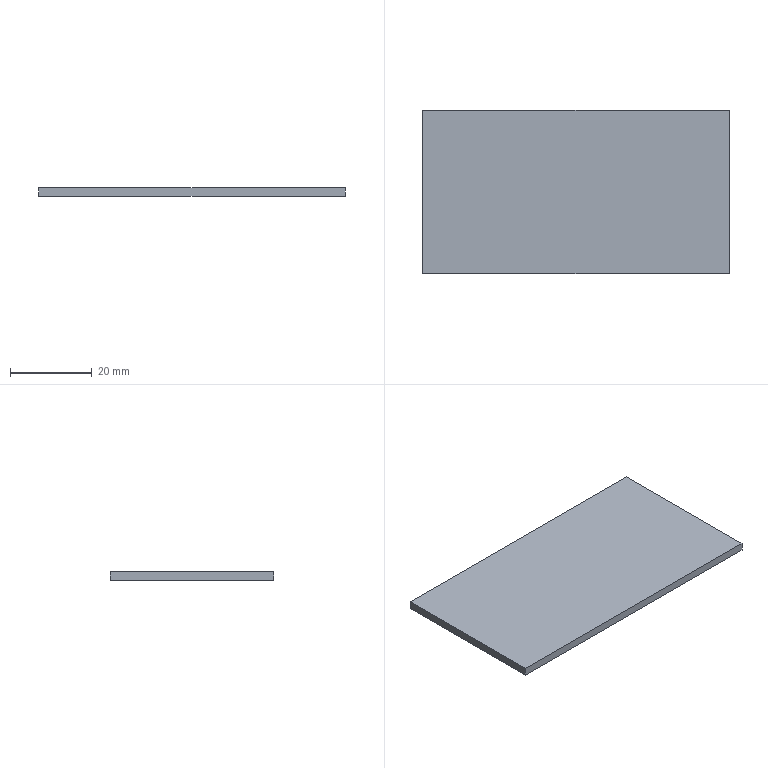Part | STEP file | Cable Carrier Seal Plate | 1 solid | 6 faces | box 75 x 40 x 2 mm | volume 6000 mm3 | plane 6
STEP:
#1=CARTESIAN_POINT('',(0.,0.,0.));
#2=DIRECTION('',(0.,0.,1.));
#3=DIRECTION('',(1.,0.,0.));
#4=AXIS2_PLACEMENT_3D('',#1,#2,#3);
#5=CARTESIAN_POINT('',(37.5,-20.,0.));
#6=VERTEX_POINT('',#5);
#7=CARTESIAN_POINT('',(37.5,20.,0.));
#8=VERTEX_POINT('',#7);
#9=CARTESIAN_POINT('',(37.5,20.,0.));
#10=DIRECTION('',(0.,1.,0.));
#11=VECTOR('',#10,1.);
#12=LINE('',#9,#11);
#13=CARTESIAN_POINT('',(37.5,20.,2.));
#14=DIRECTION('',(-1.,0.,0.));
#15=DIRECTION('',(0.,-1.,0.));
#16=AXIS2_PLACEMENT_3D('',#13,#14,#15);
#17=PLANE('',#16);
#18=CARTESIAN_POINT('',(0.,-2.));
#19=DIRECTION('',(-1.,0.));
#20=VECTOR('',#19,1.);
#21=LINE('',#18,#20);
#22=(GEOMETRIC_REPRESENTATION_CONTEXT(2)PARAMETRIC_REPRESENTATION_CONTEXT()REPRESENTATION_CONTEXT('',''));
#23=DEFINITIONAL_REPRESENTATION('',(#21),#22);
#24=PCURVE('',#17,#23);
#25=CARTESIAN_POINT('',(0.,0.,0.));
#26=DIRECTION('',(0.,0.,1.));
#27=DIRECTION('',(1.,0.,0.));
#28=AXIS2_PLACEMENT_3D('',#25,#26,#27);
#29=PLANE('',#28);
#30=CARTESIAN_POINT('',(37.5,20.));
#31=DIRECTION('',(0.,1.));
#32=VECTOR('',#31,1.);
#33=LINE('',#30,#32);
#34=(GEOMETRIC_REPRESENTATION_CONTEXT(2)PARAMETRIC_REPRESENTATION_CONTEXT()REPRESENTATION_CONTEXT('',''));
#35=DEFINITIONAL_REPRESENTATION('',(#33),#34);
#36=PCURVE('',#29,#35);
#37=SURFACE_CURVE('',#12,(#24,#36),.PCURVE_S1.);
#38=EDGE_CURVE('',#6,#8,#37,.T.);
#39=ORIENTED_EDGE('',*,*,#38,.T.);
#40=CARTESIAN_POINT('',(37.5,20.,2.));
#41=VERTEX_POINT('',#40);
#42=CARTESIAN_POINT('',(37.5,20.,2.));
#43=DIRECTION('',(0.,0.,-1.));
#44=VECTOR('',#43,1.);
#45=LINE('',#42,#44);
#46=CARTESIAN_POINT('',(0.,0.));
#47=DIRECTION('',(0.,-1.));
#48=VECTOR('',#47,1.);
#49=LINE('',#46,#48);
#50=(GEOMETRIC_REPRESENTATION_CONTEXT(2)PARAMETRIC_REPRESENTATION_CONTEXT()REPRESENTATION_CONTEXT('',''));
#51=DEFINITIONAL_REPRESENTATION('',(#49),#50);
#52=PCURVE('',#17,#51);
#53=CARTESIAN_POINT('',(-37.5,20.,2.));
#54=DIRECTION('',(0.,-1.,0.));
#55=DIRECTION('',(0.,0.,-1.));
#56=AXIS2_PLACEMENT_3D('',#53,#54,#55);
#57=PLANE('',#56);
#58=CARTESIAN_POINT('',(0.,75.));
#59=DIRECTION('',(1.,0.));
#60=VECTOR('',#59,1.);
#61=LINE('',#58,#60);
#62=(GEOMETRIC_REPRESENTATION_CONTEXT(2)PARAMETRIC_REPRESENTATION_CONTEXT()REPRESENTATION_CONTEXT('',''));
#63=DEFINITIONAL_REPRESENTATION('',(#61),#62);
#64=PCURVE('',#57,#63);
#65=SURFACE_CURVE('',#45,(#52,#64),.PCURVE_S1.);
#66=EDGE_CURVE('',#41,#8,#65,.T.);
#67=ORIENTED_EDGE('',*,*,#66,.F.);
#68=CARTESIAN_POINT('',(37.5,-20.,2.));
#69=VERTEX_POINT('',#68);
#70=CARTESIAN_POINT('',(37.5,20.,2.));
#71=DIRECTION('',(0.,1.,0.));
#72=VECTOR('',#71,1.);
#73=LINE('',#70,#72);
#74=CARTESIAN_POINT('',(0.,0.));
#75=DIRECTION('',(-1.,0.));
#76=VECTOR('',#75,1.);
#77=LINE('',#74,#76);
#78=(GEOMETRIC_REPRESENTATION_CONTEXT(2)PARAMETRIC_REPRESENTATION_CONTEXT()REPRESENTATION_CONTEXT('',''));
#79=DEFINITIONAL_REPRESENTATION('',(#77),#78);
#80=PCURVE('',#17,#79);
#81=CARTESIAN_POINT('',(0.,0.,2.));
#82=DIRECTION('',(0.,0.,1.));
#83=DIRECTION('',(1.,0.,0.));
#84=AXIS2_PLACEMENT_3D('',#81,#82,#83);
#85=PLANE('',#84);
#86=CARTESIAN_POINT('',(37.5,20.));
#87=DIRECTION('',(0.,1.));
#88=VECTOR('',#87,1.);
#89=LINE('',#86,#88);
#90=(GEOMETRIC_REPRESENTATION_CONTEXT(2)PARAMETRIC_REPRESENTATION_CONTEXT()REPRESENTATION_CONTEXT('',''));
#91=DEFINITIONAL_REPRESENTATION('',(#89),#90);
#92=PCURVE('',#85,#91);
#93=SURFACE_CURVE('',#73,(#80,#92),.PCURVE_S1.);
#94=EDGE_CURVE('',#69,#41,#93,.T.);
#95=ORIENTED_EDGE('',*,*,#94,.F.);
#96=CARTESIAN_POINT('',(37.5,-20.,2.));
#97=DIRECTION('',(0.,0.,-1.));
#98=VECTOR('',#97,1.);
#99=LINE('',#96,#98);
#100=CARTESIAN_POINT('',(40.,0.));
#101=DIRECTION('',(0.,-1.));
#102=VECTOR('',#101,1.);
#103=LINE('',#100,#102);
#104=(GEOMETRIC_REPRESENTATION_CONTEXT(2)PARAMETRIC_REPRESENTATION_CONTEXT()REPRESENTATION_CONTEXT('',''));
#105=DEFINITIONAL_REPRESENTATION('',(#103),#104);
#106=PCURVE('',#17,#105);
#107=CARTESIAN_POINT('',(-37.5,-20.,2.));
#108=DIRECTION('',(0.,1.,0.));
#109=DIRECTION('',(0.,0.,1.));
#110=AXIS2_PLACEMENT_3D('',#107,#108,#109);
#111=PLANE('',#110);
#112=CARTESIAN_POINT('',(0.,75.));
#113=DIRECTION('',(-1.,0.));
#114=VECTOR('',#113,1.);
#115=LINE('',#112,#114);
#116=(GEOMETRIC_REPRESENTATION_CONTEXT(2)PARAMETRIC_REPRESENTATION_CONTEXT()REPRESENTATION_CONTEXT('',''));
#117=DEFINITIONAL_REPRESENTATION('',(#115),#116);
#118=PCURVE('',#111,#117);
#119=SURFACE_CURVE('',#99,(#106,#118),.PCURVE_S1.);
#120=EDGE_CURVE('',#69,#6,#119,.T.);
#121=ORIENTED_EDGE('',*,*,#120,.T.);
#122=EDGE_LOOP('',(#39,#67,#95,#121));
#123=FACE_BOUND('',#122,.T.);
#124=ADVANCED_FACE('',(#123),#17,.F.);
#125=CARTESIAN_POINT('',(-37.5,20.,0.));
#126=VERTEX_POINT('',#125);
#127=CARTESIAN_POINT('',(-37.5,20.,0.));
#128=DIRECTION('',(-1.,0.,0.));
#129=VECTOR('',#128,1.);
#130=LINE('',#127,#129);
#131=CARTESIAN_POINT('',(2.,0.));
#132=DIRECTION('',(0.,-1.));
#133=VECTOR('',#132,1.);
#134=LINE('',#131,#133);
#135=(GEOMETRIC_REPRESENTATION_CONTEXT(2)PARAMETRIC_REPRESENTATION_CONTEXT()REPRESENTATION_CONTEXT('',''));
#136=DEFINITIONAL_REPRESENTATION('',(#134),#135);
#137=PCURVE('',#57,#136);
#138=CARTESIAN_POINT('',(-37.5,20.));
#139=DIRECTION('',(-1.,0.));
#140=VECTOR('',#139,1.);
#141=LINE('',#138,#140);
#142=(GEOMETRIC_REPRESENTATION_CONTEXT(2)PARAMETRIC_REPRESENTATION_CONTEXT()REPRESENTATION_CONTEXT('',''));
#143=DEFINITIONAL_REPRESENTATION('',(#141),#142);
#144=PCURVE('',#29,#143);
#145=SURFACE_CURVE('',#130,(#137,#144),.PCURVE_S1.);
#146=EDGE_CURVE('',#8,#126,#145,.T.);
#147=ORIENTED_EDGE('',*,*,#146,.T.);
#148=CARTESIAN_POINT('',(-37.5,20.,2.));
#149=VERTEX_POINT('',#148);
#150=CARTESIAN_POINT('',(-37.5,20.,2.));
#151=DIRECTION('',(0.,0.,-1.));
#152=VECTOR('',#151,1.);
#153=LINE('',#150,#152);
#154=CARTESIAN_POINT('',(0.,0.));
#155=DIRECTION('',(1.,0.));
#156=VECTOR('',#155,1.);
#157=LINE('',#154,#156);
#158=(GEOMETRIC_REPRESENTATION_CONTEXT(2)PARAMETRIC_REPRESENTATION_CONTEXT()REPRESENTATION_CONTEXT('',''));
#159=DEFINITIONAL_REPRESENTATION('',(#157),#158);
#160=PCURVE('',#57,#159);
#161=CARTESIAN_POINT('',(-37.5,20.,2.));
#162=DIRECTION('',(1.,0.,0.));
#163=DIRECTION('',(0.,1.,0.));
#164=AXIS2_PLACEMENT_3D('',#161,#162,#163);
#165=PLANE('',#164);
#166=CARTESIAN_POINT('',(0.,0.));
#167=DIRECTION('',(0.,-1.));
#168=VECTOR('',#167,1.);
#169=LINE('',#166,#168);
#170=(GEOMETRIC_REPRESENTATION_CONTEXT(2)PARAMETRIC_REPRESENTATION_CONTEXT()REPRESENTATION_CONTEXT('',''));
#171=DEFINITIONAL_REPRESENTATION('',(#169),#170);
#172=PCURVE('',#165,#171);
#173=SURFACE_CURVE('',#153,(#160,#172),.PCURVE_S1.);
#174=EDGE_CURVE('',#149,#126,#173,.T.);
#175=ORIENTED_EDGE('',*,*,#174,.F.);
#176=CARTESIAN_POINT('',(-37.5,20.,2.));
#177=DIRECTION('',(-1.,0.,0.));
#178=VECTOR('',#177,1.);
#179=LINE('',#176,#178);
#180=CARTESIAN_POINT('',(0.,0.));
#181=DIRECTION('',(0.,-1.));
#182=VECTOR('',#181,1.);
#183=LINE('',#180,#182);
#184=(GEOMETRIC_REPRESENTATION_CONTEXT(2)PARAMETRIC_REPRESENTATION_CONTEXT()REPRESENTATION_CONTEXT('',''));
#185=DEFINITIONAL_REPRESENTATION('',(#183),#184);
#186=PCURVE('',#57,#185);
#187=CARTESIAN_POINT('',(-37.5,20.));
#188=DIRECTION('',(-1.,0.));
#189=VECTOR('',#188,1.);
#190=LINE('',#187,#189);
#191=(GEOMETRIC_REPRESENTATION_CONTEXT(2)PARAMETRIC_REPRESENTATION_CONTEXT()REPRESENTATION_CONTEXT('',''));
#192=DEFINITIONAL_REPRESENTATION('',(#190),#191);
#193=PCURVE('',#85,#192);
#194=SURFACE_CURVE('',#179,(#186,#193),.PCURVE_S1.);
#195=EDGE_CURVE('',#41,#149,#194,.T.);
#196=ORIENTED_EDGE('',*,*,#195,.F.);
#197=ORIENTED_EDGE('',*,*,#66,.T.);
#198=EDGE_LOOP('',(#147,#175,#196,#197));
#199=FACE_BOUND('',#198,.T.);
#200=ADVANCED_FACE('',(#199),#57,.F.);
#201=CARTESIAN_POINT('',(-37.5,-20.,0.));
#202=VERTEX_POINT('',#201);
#203=CARTESIAN_POINT('',(-37.5,20.,0.));
#204=DIRECTION('',(0.,-1.,0.));
#205=VECTOR('',#204,1.);
#206=LINE('',#203,#205);
#207=CARTESIAN_POINT('',(0.,-2.));
#208=DIRECTION('',(-1.,0.));
#209=VECTOR('',#208,1.);
#210=LINE('',#207,#209);
#211=(GEOMETRIC_REPRESENTATION_CONTEXT(2)PARAMETRIC_REPRESENTATION_CONTEXT()REPRESENTATION_CONTEXT('',''));
#212=DEFINITIONAL_REPRESENTATION('',(#210),#211);
#213=PCURVE('',#165,#212);
#214=CARTESIAN_POINT('',(-37.5,20.));
#215=DIRECTION('',(0.,-1.));
#216=VECTOR('',#215,1.);
#217=LINE('',#214,#216);
#218=(GEOMETRIC_REPRESENTATION_CONTEXT(2)PARAMETRIC_REPRESENTATION_CONTEXT()REPRESENTATION_CONTEXT('',''));
#219=DEFINITIONAL_REPRESENTATION('',(#217),#218);
#220=PCURVE('',#29,#219);
#221=SURFACE_CURVE('',#206,(#213,#220),.PCURVE_S1.);
#222=EDGE_CURVE('',#126,#202,#221,.T.);
#223=ORIENTED_EDGE('',*,*,#222,.T.);
#224=CARTESIAN_POINT('',(-37.5,-20.,2.));
#225=VERTEX_POINT('',#224);
#226=CARTESIAN_POINT('',(-37.5,-20.,2.));
#227=DIRECTION('',(0.,0.,-1.));
#228=VECTOR('',#227,1.);
#229=LINE('',#226,#228);
#230=CARTESIAN_POINT('',(-40.,0.));
#231=DIRECTION('',(0.,-1.));
#232=VECTOR('',#231,1.);
#233=LINE('',#230,#232);
#234=(GEOMETRIC_REPRESENTATION_CONTEXT(2)PARAMETRIC_REPRESENTATION_CONTEXT()REPRESENTATION_CONTEXT('',''));
#235=DEFINITIONAL_REPRESENTATION('',(#233),#234);
#236=PCURVE('',#165,#235);
#237=CARTESIAN_POINT('',(0.,0.));
#238=DIRECTION('',(-1.,0.));
#239=VECTOR('',#238,1.);
#240=LINE('',#237,#239);
#241=(GEOMETRIC_REPRESENTATION_CONTEXT(2)PARAMETRIC_REPRESENTATION_CONTEXT()REPRESENTATION_CONTEXT('',''));
#242=DEFINITIONAL_REPRESENTATION('',(#240),#241);
#243=PCURVE('',#111,#242);
#244=SURFACE_CURVE('',#229,(#236,#243),.PCURVE_S1.);
#245=EDGE_CURVE('',#225,#202,#244,.T.);
#246=ORIENTED_EDGE('',*,*,#245,.F.);
#247=CARTESIAN_POINT('',(-37.5,20.,2.));
#248=DIRECTION('',(0.,-1.,0.));
#249=VECTOR('',#248,1.);
#250=LINE('',#247,#249);
#251=CARTESIAN_POINT('',(0.,0.));
#252=DIRECTION('',(-1.,0.));
#253=VECTOR('',#252,1.);
#254=LINE('',#251,#253);
#255=(GEOMETRIC_REPRESENTATION_CONTEXT(2)PARAMETRIC_REPRESENTATION_CONTEXT()REPRESENTATION_CONTEXT('',''));
#256=DEFINITIONAL_REPRESENTATION('',(#254),#255);
#257=PCURVE('',#165,#256);
#258=CARTESIAN_POINT('',(-37.5,20.));
#259=DIRECTION('',(0.,-1.));
#260=VECTOR('',#259,1.);
#261=LINE('',#258,#260);
#262=(GEOMETRIC_REPRESENTATION_CONTEXT(2)PARAMETRIC_REPRESENTATION_CONTEXT()REPRESENTATION_CONTEXT('',''));
#263=DEFINITIONAL_REPRESENTATION('',(#261),#262);
#264=PCURVE('',#85,#263);
#265=SURFACE_CURVE('',#250,(#257,#264),.PCURVE_S1.);
#266=EDGE_CURVE('',#149,#225,#265,.T.);
#267=ORIENTED_EDGE('',*,*,#266,.F.);
#268=ORIENTED_EDGE('',*,*,#174,.T.);
#269=EDGE_LOOP('',(#223,#246,#267,#268));
#270=FACE_BOUND('',#269,.T.);
#271=ADVANCED_FACE('',(#270),#165,.F.);
#272=CARTESIAN_POINT('',(-37.5,-20.,0.));
#273=DIRECTION('',(1.,0.,0.));
#274=VECTOR('',#273,1.);
#275=LINE('',#272,#274);
#276=CARTESIAN_POINT('',(-2.,0.));
#277=DIRECTION('',(0.,1.));
#278=VECTOR('',#277,1.);
#279=LINE('',#276,#278);
#280=(GEOMETRIC_REPRESENTATION_CONTEXT(2)PARAMETRIC_REPRESENTATION_CONTEXT()REPRESENTATION_CONTEXT('',''));
#281=DEFINITIONAL_REPRESENTATION('',(#279),#280);
#282=PCURVE('',#111,#281);
#283=CARTESIAN_POINT('',(-37.5,-20.));
#284=DIRECTION('',(1.,0.));
#285=VECTOR('',#284,1.);
#286=LINE('',#283,#285);
#287=(GEOMETRIC_REPRESENTATION_CONTEXT(2)PARAMETRIC_REPRESENTATION_CONTEXT()REPRESENTATION_CONTEXT('',''));
#288=DEFINITIONAL_REPRESENTATION('',(#286),#287);
#289=PCURVE('',#29,#288);
#290=SURFACE_CURVE('',#275,(#282,#289),.PCURVE_S1.);
#291=EDGE_CURVE('',#202,#6,#290,.T.);
#292=ORIENTED_EDGE('',*,*,#291,.T.);
#293=ORIENTED_EDGE('',*,*,#120,.F.);
#294=CARTESIAN_POINT('',(-37.5,-20.,2.));
#295=DIRECTION('',(1.,0.,0.));
#296=VECTOR('',#295,1.);
#297=LINE('',#294,#296);
#298=CARTESIAN_POINT('',(0.,0.));
#299=DIRECTION('',(0.,1.));
#300=VECTOR('',#299,1.);
#301=LINE('',#298,#300);
#302=(GEOMETRIC_REPRESENTATION_CONTEXT(2)PARAMETRIC_REPRESENTATION_CONTEXT()REPRESENTATION_CONTEXT('',''));
#303=DEFINITIONAL_REPRESENTATION('',(#301),#302);
#304=PCURVE('',#111,#303);
#305=CARTESIAN_POINT('',(-37.5,-20.));
#306=DIRECTION('',(1.,0.));
#307=VECTOR('',#306,1.);
#308=LINE('',#305,#307);
#309=(GEOMETRIC_REPRESENTATION_CONTEXT(2)PARAMETRIC_REPRESENTATION_CONTEXT()REPRESENTATION_CONTEXT('',''));
#310=DEFINITIONAL_REPRESENTATION('',(#308),#309);
#311=PCURVE('',#85,#310);
#312=SURFACE_CURVE('',#297,(#304,#311),.PCURVE_S1.);
#313=EDGE_CURVE('',#225,#69,#312,.T.);
#314=ORIENTED_EDGE('',*,*,#313,.F.);
#315=ORIENTED_EDGE('',*,*,#245,.T.);
#316=EDGE_LOOP('',(#292,#293,#314,#315));
#317=FACE_BOUND('',#316,.T.);
#318=ADVANCED_FACE('',(#317),#111,.F.);
#319=ORIENTED_EDGE('',*,*,#94,.T.);
#320=ORIENTED_EDGE('',*,*,#195,.T.);
#321=ORIENTED_EDGE('',*,*,#266,.T.);
#322=ORIENTED_EDGE('',*,*,#313,.T.);
#323=EDGE_LOOP('',(#319,#320,#321,#322));
#324=FACE_BOUND('',#323,.T.);
#325=ADVANCED_FACE('',(#324),#85,.T.);
#326=ORIENTED_EDGE('',*,*,#38,.F.);
#327=ORIENTED_EDGE('',*,*,#291,.F.);
#328=ORIENTED_EDGE('',*,*,#222,.F.);
#329=ORIENTED_EDGE('',*,*,#146,.F.);
#330=EDGE_LOOP('',(#326,#327,#328,#329));
#331=FACE_BOUND('',#330,.T.);
#332=ADVANCED_FACE('',(#331),#29,.F.);
#333=CLOSED_SHELL('',(#124,#200,#271,#318,#325,#332));
#334=MANIFOLD_SOLID_BREP('',#333);
#335=(LENGTH_UNIT()NAMED_UNIT(*)SI_UNIT(.MILLI.,.METRE.));
#336=UNCERTAINTY_MEASURE_WITH_UNIT(LENGTH_MEASURE(0.0000001),#335,'','');
#337=(NAMED_UNIT(*)PLANE_ANGLE_UNIT()SI_UNIT($,.RADIAN.));
#338=(NAMED_UNIT(*)SI_UNIT($,.STERADIAN.)SOLID_ANGLE_UNIT());
#339=(GEOMETRIC_REPRESENTATION_CONTEXT(3)GLOBAL_UNCERTAINTY_ASSIGNED_CONTEXT((#336))GLOBAL_UNIT_ASSIGNED_CONTEXT((#335,#337,#338))REPRESENTATION_CONTEXT('',''));
#340=ADVANCED_BREP_SHAPE_REPRESENTATION('',(#4,#334),#339);